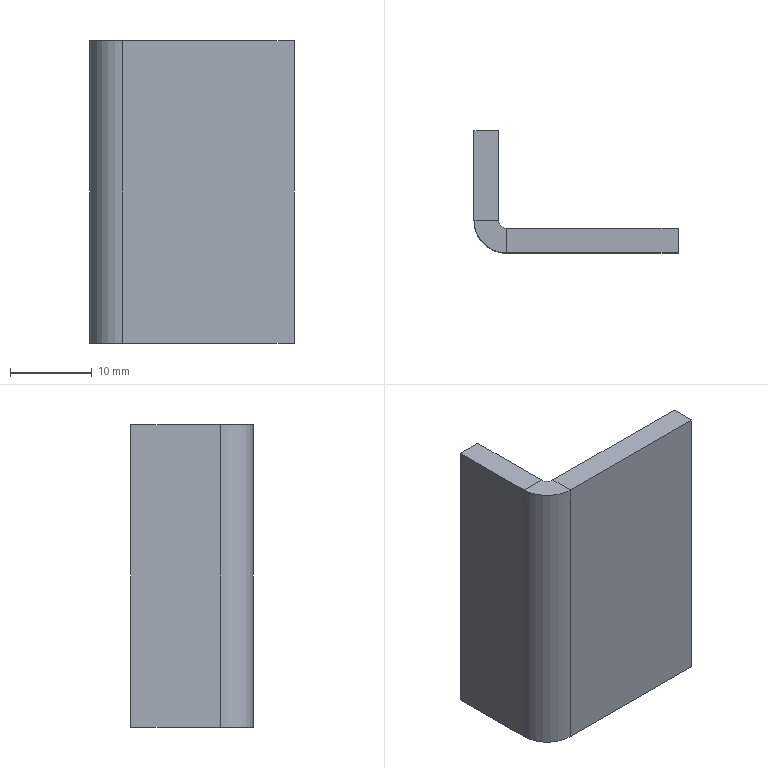Part | SolidWorks | features BaseBody 1 | 1 solid | 14 faces | box 25 x 15 x 37 mm | volume 3988 mm3 | plane 12 | cylinder 2 | commonest cylinder face diameters 2 x1 8 x1
STEP:
#1=CARTESIAN_POINT('',(4.,0.,18.5));
#2=VERTEX_POINT('',#1);
#3=CARTESIAN_POINT('',(25.,0.,18.5));
#4=VERTEX_POINT('',#3);
#5=CARTESIAN_POINT('',(0.,0.,18.5));
#6=DIRECTION('',(1.,0.,0.));
#7=VECTOR('',#6,1000.);
#8=LINE('',#5,#7);
#9=EDGE_CURVE('',#2,#4,#8,.T.);
#10=ORIENTED_EDGE('',*,*,#9,.T.);
#11=CARTESIAN_POINT('',(25.,3.,18.5));
#12=VERTEX_POINT('',#11);
#13=CARTESIAN_POINT('',(25.,3.,18.5));
#14=DIRECTION('',(0.,-1.,0.));
#15=VECTOR('',#14,1000.);
#16=LINE('',#13,#15);
#17=EDGE_CURVE('',#12,#4,#16,.T.);
#18=ORIENTED_EDGE('',*,*,#17,.F.);
#19=CARTESIAN_POINT('',(4.,3.,18.5));
#20=VERTEX_POINT('',#19);
#21=CARTESIAN_POINT('',(0.,3.,18.5));
#22=DIRECTION('',(1.,0.,0.));
#23=VECTOR('',#22,1000.);
#24=LINE('',#21,#23);
#25=EDGE_CURVE('',#20,#12,#24,.T.);
#26=ORIENTED_EDGE('',*,*,#25,.F.);
#27=CARTESIAN_POINT('',(4.,3.,18.5));
#28=DIRECTION('',(0.,-1.,0.));
#29=VECTOR('',#28,1000.);
#30=LINE('',#27,#29);
#31=EDGE_CURVE('',#20,#2,#30,.T.);
#32=ORIENTED_EDGE('',*,*,#31,.T.);
#33=EDGE_LOOP('',(#10,#18,#26,#32));
#34=FACE_OUTER_BOUND('',#33,.T.);
#35=CARTESIAN_POINT('',(4.,4.,18.5));
#36=DIRECTION('',(0.,0.,1.));
#37=DIRECTION('',(1.,0.,0.));
#38=AXIS2_PLACEMENT_3D('',#35,#36,#37);
#39=PLANE('',#38);
#40=ADVANCED_FACE('',(#34),#39,.T.);
#41=CARTESIAN_POINT('',(3.,15.,-18.5));
#42=VERTEX_POINT('',#41);
#43=CARTESIAN_POINT('',(3.,4.,-18.5));
#44=VERTEX_POINT('',#43);
#45=CARTESIAN_POINT('',(3.,0.,-18.5));
#46=DIRECTION('',(0.,-1.,0.));
#47=VECTOR('',#46,1000.);
#48=LINE('',#45,#47);
#49=EDGE_CURVE('',#42,#44,#48,.T.);
#50=ORIENTED_EDGE('',*,*,#49,.T.);
#51=CARTESIAN_POINT('',(0.,4.,-18.5));
#52=VERTEX_POINT('',#51);
#53=CARTESIAN_POINT('',(3.,4.,-18.5));
#54=DIRECTION('',(-1.,0.,0.));
#55=VECTOR('',#54,1000.);
#56=LINE('',#53,#55);
#57=EDGE_CURVE('',#44,#52,#56,.T.);
#58=ORIENTED_EDGE('',*,*,#57,.T.);
#59=CARTESIAN_POINT('',(0.,15.,-18.5));
#60=VERTEX_POINT('',#59);
#61=CARTESIAN_POINT('',(0.,0.,-18.5));
#62=DIRECTION('',(0.,-1.,0.));
#63=VECTOR('',#62,1000.);
#64=LINE('',#61,#63);
#65=EDGE_CURVE('',#60,#52,#64,.T.);
#66=ORIENTED_EDGE('',*,*,#65,.F.);
#67=CARTESIAN_POINT('',(0.,15.,-18.5));
#68=DIRECTION('',(1.,0.,0.));
#69=VECTOR('',#68,1000.);
#70=LINE('',#67,#69);
#71=EDGE_CURVE('',#60,#42,#70,.T.);
#72=ORIENTED_EDGE('',*,*,#71,.T.);
#73=EDGE_LOOP('',(#50,#58,#66,#72));
#74=FACE_OUTER_BOUND('',#73,.T.);
#75=CARTESIAN_POINT('',(4.,4.,-18.5));
#76=DIRECTION('',(0.,0.,1.));
#77=DIRECTION('',(1.,0.,0.));
#78=AXIS2_PLACEMENT_3D('',#75,#76,#77);
#79=PLANE('',#78);
#80=ADVANCED_FACE('',(#74),#79,.F.);
#81=ORIENTED_EDGE('',*,*,#17,.T.);
#82=CARTESIAN_POINT('',(25.,0.,-18.5));
#83=VERTEX_POINT('',#82);
#84=CARTESIAN_POINT('',(25.,0.,-18.5));
#85=DIRECTION('',(0.,0.,1.));
#86=VECTOR('',#85,1000.);
#87=LINE('',#84,#86);
#88=EDGE_CURVE('',#83,#4,#87,.T.);
#89=ORIENTED_EDGE('',*,*,#88,.F.);
#90=CARTESIAN_POINT('',(25.,3.,-18.5));
#91=VERTEX_POINT('',#90);
#92=CARTESIAN_POINT('',(25.,3.,-18.5));
#93=DIRECTION('',(0.,-1.,0.));
#94=VECTOR('',#93,1000.);
#95=LINE('',#92,#94);
#96=EDGE_CURVE('',#91,#83,#95,.T.);
#97=ORIENTED_EDGE('',*,*,#96,.F.);
#98=CARTESIAN_POINT('',(25.,3.,-18.5));
#99=DIRECTION('',(0.,0.,1.));
#100=VECTOR('',#99,1000.);
#101=LINE('',#98,#100);
#102=EDGE_CURVE('',#91,#12,#101,.T.);
#103=ORIENTED_EDGE('',*,*,#102,.T.);
#104=EDGE_LOOP('',(#81,#89,#97,#103));
#105=FACE_OUTER_BOUND('',#104,.T.);
#106=CARTESIAN_POINT('',(25.,3.,-18.5));
#107=DIRECTION('',(-1.,0.,0.));
#108=DIRECTION('',(0.,0.,1.));
#109=AXIS2_PLACEMENT_3D('',#106,#107,#108);
#110=PLANE('',#109);
#111=ADVANCED_FACE('',(#105),#110,.F.);
#112=ORIENTED_EDGE('',*,*,#25,.T.);
#113=ORIENTED_EDGE('',*,*,#102,.F.);
#114=CARTESIAN_POINT('',(4.,3.,-18.5));
#115=VERTEX_POINT('',#114);
#116=CARTESIAN_POINT('',(0.,3.,-18.5));
#117=DIRECTION('',(1.,0.,0.));
#118=VECTOR('',#117,1000.);
#119=LINE('',#116,#118);
#120=EDGE_CURVE('',#115,#91,#119,.T.);
#121=ORIENTED_EDGE('',*,*,#120,.F.);
#122=CARTESIAN_POINT('',(4.,3.,-18.5));
#123=DIRECTION('',(0.,0.,1.));
#124=VECTOR('',#123,1000.);
#125=LINE('',#122,#124);
#126=EDGE_CURVE('',#115,#20,#125,.T.);
#127=ORIENTED_EDGE('',*,*,#126,.T.);
#128=EDGE_LOOP('',(#112,#113,#121,#127));
#129=FACE_OUTER_BOUND('',#128,.T.);
#130=CARTESIAN_POINT('',(0.,3.,-18.5));
#131=DIRECTION('',(0.,-1.,0.));
#132=DIRECTION('',(0.,0.,-1.));
#133=AXIS2_PLACEMENT_3D('',#130,#131,#132);
#134=PLANE('',#133);
#135=ADVANCED_FACE('',(#129),#134,.F.);
#136=CARTESIAN_POINT('',(3.,4.,18.5));
#137=VERTEX_POINT('',#136);
#138=CARTESIAN_POINT('',(4.,4.,18.5));
#139=DIRECTION('',(0.,0.,1.));
#140=DIRECTION('',(1.,0.,0.));
#141=AXIS2_PLACEMENT_3D('',#138,#139,#140);
#142=CIRCLE('',#141,1.);
#143=EDGE_CURVE('',#137,#20,#142,.T.);
#144=ORIENTED_EDGE('',*,*,#143,.T.);
#145=ORIENTED_EDGE('',*,*,#126,.F.);
#146=CARTESIAN_POINT('',(4.,4.,-18.5));
#147=DIRECTION('',(0.,0.,1.));
#148=DIRECTION('',(1.,0.,0.));
#149=AXIS2_PLACEMENT_3D('',#146,#147,#148);
#150=CIRCLE('',#149,1.);
#151=EDGE_CURVE('',#44,#115,#150,.T.);
#152=ORIENTED_EDGE('',*,*,#151,.F.);
#153=CARTESIAN_POINT('',(3.,4.,-18.5));
#154=DIRECTION('',(0.,0.,1.));
#155=VECTOR('',#154,1000.);
#156=LINE('',#153,#155);
#157=EDGE_CURVE('',#44,#137,#156,.T.);
#158=ORIENTED_EDGE('',*,*,#157,.T.);
#159=EDGE_LOOP('',(#144,#145,#152,#158));
#160=FACE_OUTER_BOUND('',#159,.T.);
#161=CARTESIAN_POINT('',(4.,4.,-18.5));
#162=DIRECTION('',(0.,0.,1.));
#163=DIRECTION('',(1.,0.,0.));
#164=AXIS2_PLACEMENT_3D('',#161,#162,#163);
#165=CYLINDRICAL_SURFACE('',#164,1.);
#166=ADVANCED_FACE('',(#160),#165,.F.);
#167=CARTESIAN_POINT('',(3.,15.,18.5));
#168=VERTEX_POINT('',#167);
#169=CARTESIAN_POINT('',(3.,0.,18.5));
#170=DIRECTION('',(0.,-1.,0.));
#171=VECTOR('',#170,1000.);
#172=LINE('',#169,#171);
#173=EDGE_CURVE('',#168,#137,#172,.T.);
#174=ORIENTED_EDGE('',*,*,#173,.T.);
#175=ORIENTED_EDGE('',*,*,#157,.F.);
#176=ORIENTED_EDGE('',*,*,#49,.F.);
#177=CARTESIAN_POINT('',(3.,15.,-18.5));
#178=DIRECTION('',(0.,0.,1.));
#179=VECTOR('',#178,1000.);
#180=LINE('',#177,#179);
#181=EDGE_CURVE('',#42,#168,#180,.T.);
#182=ORIENTED_EDGE('',*,*,#181,.T.);
#183=EDGE_LOOP('',(#174,#175,#176,#182));
#184=FACE_OUTER_BOUND('',#183,.T.);
#185=CARTESIAN_POINT('',(3.,0.,-18.5));
#186=DIRECTION('',(-1.,0.,0.));
#187=DIRECTION('',(0.,0.,1.));
#188=AXIS2_PLACEMENT_3D('',#185,#186,#187);
#189=PLANE('',#188);
#190=ADVANCED_FACE('',(#184),#189,.F.);
#191=CARTESIAN_POINT('',(0.,15.,18.5));
#192=VERTEX_POINT('',#191);
#193=CARTESIAN_POINT('',(0.,15.,18.5));
#194=DIRECTION('',(1.,0.,0.));
#195=VECTOR('',#194,1000.);
#196=LINE('',#193,#195);
#197=EDGE_CURVE('',#192,#168,#196,.T.);
#198=ORIENTED_EDGE('',*,*,#197,.T.);
#199=ORIENTED_EDGE('',*,*,#181,.F.);
#200=ORIENTED_EDGE('',*,*,#71,.F.);
#201=CARTESIAN_POINT('',(0.,15.,-18.5));
#202=DIRECTION('',(0.,0.,1.));
#203=VECTOR('',#202,1000.);
#204=LINE('',#201,#203);
#205=EDGE_CURVE('',#60,#192,#204,.T.);
#206=ORIENTED_EDGE('',*,*,#205,.T.);
#207=EDGE_LOOP('',(#198,#199,#200,#206));
#208=FACE_OUTER_BOUND('',#207,.T.);
#209=CARTESIAN_POINT('',(0.,15.,-18.5));
#210=DIRECTION('',(0.,-1.,0.));
#211=DIRECTION('',(0.,0.,-1.));
#212=AXIS2_PLACEMENT_3D('',#209,#210,#211);
#213=PLANE('',#212);
#214=ADVANCED_FACE('',(#208),#213,.F.);
#215=CARTESIAN_POINT('',(0.,4.,18.5));
#216=VERTEX_POINT('',#215);
#217=CARTESIAN_POINT('',(0.,0.,18.5));
#218=DIRECTION('',(0.,-1.,0.));
#219=VECTOR('',#218,1000.);
#220=LINE('',#217,#219);
#221=EDGE_CURVE('',#192,#216,#220,.T.);
#222=ORIENTED_EDGE('',*,*,#221,.F.);
#223=ORIENTED_EDGE('',*,*,#205,.F.);
#224=ORIENTED_EDGE('',*,*,#65,.T.);
#225=CARTESIAN_POINT('',(0.,4.,-18.5));
#226=DIRECTION('',(0.,0.,1.));
#227=VECTOR('',#226,1000.);
#228=LINE('',#225,#227);
#229=EDGE_CURVE('',#52,#216,#228,.T.);
#230=ORIENTED_EDGE('',*,*,#229,.T.);
#231=EDGE_LOOP('',(#222,#223,#224,#230));
#232=FACE_OUTER_BOUND('',#231,.T.);
#233=CARTESIAN_POINT('',(0.,0.,-18.5));
#234=DIRECTION('',(-1.,0.,0.));
#235=DIRECTION('',(0.,0.,1.));
#236=AXIS2_PLACEMENT_3D('',#233,#234,#235);
#237=PLANE('',#236);
#238=ADVANCED_FACE('',(#232),#237,.T.);
#239=CARTESIAN_POINT('',(4.,4.,18.5));
#240=DIRECTION('',(0.,0.,1.));
#241=DIRECTION('',(-1.,0.,0.));
#242=AXIS2_PLACEMENT_3D('',#239,#240,#241);
#243=CIRCLE('',#242,4.);
#244=EDGE_CURVE('',#216,#2,#243,.T.);
#245=ORIENTED_EDGE('',*,*,#244,.F.);
#246=ORIENTED_EDGE('',*,*,#229,.F.);
#247=CARTESIAN_POINT('',(4.,0.,-18.5));
#248=VERTEX_POINT('',#247);
#249=CARTESIAN_POINT('',(4.,4.,-18.5));
#250=DIRECTION('',(0.,0.,1.));
#251=DIRECTION('',(-1.,0.,0.));
#252=AXIS2_PLACEMENT_3D('',#249,#250,#251);
#253=CIRCLE('',#252,4.);
#254=EDGE_CURVE('',#52,#248,#253,.T.);
#255=ORIENTED_EDGE('',*,*,#254,.T.);
#256=CARTESIAN_POINT('',(4.,0.,-18.5));
#257=DIRECTION('',(0.,0.,1.));
#258=VECTOR('',#257,1000.);
#259=LINE('',#256,#258);
#260=EDGE_CURVE('',#248,#2,#259,.T.);
#261=ORIENTED_EDGE('',*,*,#260,.T.);
#262=EDGE_LOOP('',(#245,#246,#255,#261));
#263=FACE_OUTER_BOUND('',#262,.T.);
#264=CARTESIAN_POINT('',(4.,4.,-18.5));
#265=DIRECTION('',(0.,0.,1.));
#266=DIRECTION('',(1.,0.,0.));
#267=AXIS2_PLACEMENT_3D('',#264,#265,#266);
#268=CYLINDRICAL_SURFACE('',#267,4.);
#269=ADVANCED_FACE('',(#263),#268,.T.);
#270=ORIENTED_EDGE('',*,*,#9,.F.);
#271=ORIENTED_EDGE('',*,*,#260,.F.);
#272=CARTESIAN_POINT('',(0.,0.,-18.5));
#273=DIRECTION('',(1.,0.,0.));
#274=VECTOR('',#273,1000.);
#275=LINE('',#272,#274);
#276=EDGE_CURVE('',#248,#83,#275,.T.);
#277=ORIENTED_EDGE('',*,*,#276,.T.);
#278=ORIENTED_EDGE('',*,*,#88,.T.);
#279=EDGE_LOOP('',(#270,#271,#277,#278));
#280=FACE_OUTER_BOUND('',#279,.T.);
#281=CARTESIAN_POINT('',(0.,0.,-18.5));
#282=DIRECTION('',(0.,-1.,0.));
#283=DIRECTION('',(0.,0.,-1.));
#284=AXIS2_PLACEMENT_3D('',#281,#282,#283);
#285=PLANE('',#284);
#286=ADVANCED_FACE('',(#280),#285,.T.);
#287=ORIENTED_EDGE('',*,*,#221,.T.);
#288=CARTESIAN_POINT('',(0.,4.,18.5));
#289=DIRECTION('',(1.,0.,0.));
#290=VECTOR('',#289,1000.);
#291=LINE('',#288,#290);
#292=EDGE_CURVE('',#216,#137,#291,.T.);
#293=ORIENTED_EDGE('',*,*,#292,.T.);
#294=ORIENTED_EDGE('',*,*,#173,.F.);
#295=ORIENTED_EDGE('',*,*,#197,.F.);
#296=EDGE_LOOP('',(#287,#293,#294,#295));
#297=FACE_OUTER_BOUND('',#296,.T.);
#298=CARTESIAN_POINT('',(4.,3.,18.5));
#299=DIRECTION('',(0.,0.,1.));
#300=DIRECTION('',(1.,0.,0.));
#301=AXIS2_PLACEMENT_3D('',#298,#299,#300);
#302=PLANE('',#301);
#303=ADVANCED_FACE('',(#297),#302,.T.);
#304=ORIENTED_EDGE('',*,*,#292,.F.);
#305=ORIENTED_EDGE('',*,*,#244,.T.);
#306=ORIENTED_EDGE('',*,*,#31,.F.);
#307=ORIENTED_EDGE('',*,*,#143,.F.);
#308=EDGE_LOOP('',(#304,#305,#306,#307));
#309=FACE_OUTER_BOUND('',#308,.T.);
#310=CARTESIAN_POINT('',(0.,4.,18.5));
#311=DIRECTION('',(0.,0.,1.));
#312=DIRECTION('',(1.,0.,0.));
#313=AXIS2_PLACEMENT_3D('',#310,#311,#312);
#314=PLANE('',#313);
#315=ADVANCED_FACE('',(#309),#314,.T.);
#316=ORIENTED_EDGE('',*,*,#276,.F.);
#317=CARTESIAN_POINT('',(4.,0.,-18.5));
#318=DIRECTION('',(0.,1.,0.));
#319=VECTOR('',#318,1000.);
#320=LINE('',#317,#319);
#321=EDGE_CURVE('',#248,#115,#320,.T.);
#322=ORIENTED_EDGE('',*,*,#321,.T.);
#323=ORIENTED_EDGE('',*,*,#120,.T.);
#324=ORIENTED_EDGE('',*,*,#96,.T.);
#325=EDGE_LOOP('',(#316,#322,#323,#324));
#326=FACE_OUTER_BOUND('',#325,.T.);
#327=CARTESIAN_POINT('',(3.,4.,-18.5));
#328=DIRECTION('',(0.,0.,-1.));
#329=DIRECTION('',(0.,-1.,0.));
#330=AXIS2_PLACEMENT_3D('',#327,#328,#329);
#331=PLANE('',#330);
#332=ADVANCED_FACE('',(#326),#331,.T.);
#333=ORIENTED_EDGE('',*,*,#321,.F.);
#334=ORIENTED_EDGE('',*,*,#254,.F.);
#335=ORIENTED_EDGE('',*,*,#57,.F.);
#336=ORIENTED_EDGE('',*,*,#151,.T.);
#337=EDGE_LOOP('',(#333,#334,#335,#336));
#338=FACE_OUTER_BOUND('',#337,.T.);
#339=CARTESIAN_POINT('',(4.,0.,-18.5));
#340=DIRECTION('',(0.,0.,-1.));
#341=DIRECTION('',(0.,-1.,0.));
#342=AXIS2_PLACEMENT_3D('',#339,#340,#341);
#343=PLANE('',#342);
#344=ADVANCED_FACE('',(#338),#343,.T.);
#345=CLOSED_SHELL('',(#40,#80,#111,#135,#166,#190,#214,#238,#269,#286,#303,#315,#332,#344));
#346=MANIFOLD_SOLID_BREP('',#345);
#347=CARTESIAN_POINT('',(0.,0.,0.));
#348=DIRECTION('',(0.,0.,1.));
#349=DIRECTION('',(1.,0.,0.));
#350=AXIS2_PLACEMENT_3D('',#347,#348,#349);
#351=(LENGTH_UNIT()NAMED_UNIT(*)SI_UNIT(.MILLI.,.METRE.));
#352=UNCERTAINTY_MEASURE_WITH_UNIT(LENGTH_MEASURE(0.00001),#351,'','');
#353=(NAMED_UNIT(*)PLANE_ANGLE_UNIT()SI_UNIT($,.RADIAN.));
#354=(NAMED_UNIT(*)SI_UNIT($,.STERADIAN.)SOLID_ANGLE_UNIT());
#355=(GEOMETRIC_REPRESENTATION_CONTEXT(3)GLOBAL_UNCERTAINTY_ASSIGNED_CONTEXT((#352))GLOBAL_UNIT_ASSIGNED_CONTEXT((#351,#353,#354))REPRESENTATION_CONTEXT('',''));
#356=ADVANCED_BREP_SHAPE_REPRESENTATION('',(#346,#350),#355);